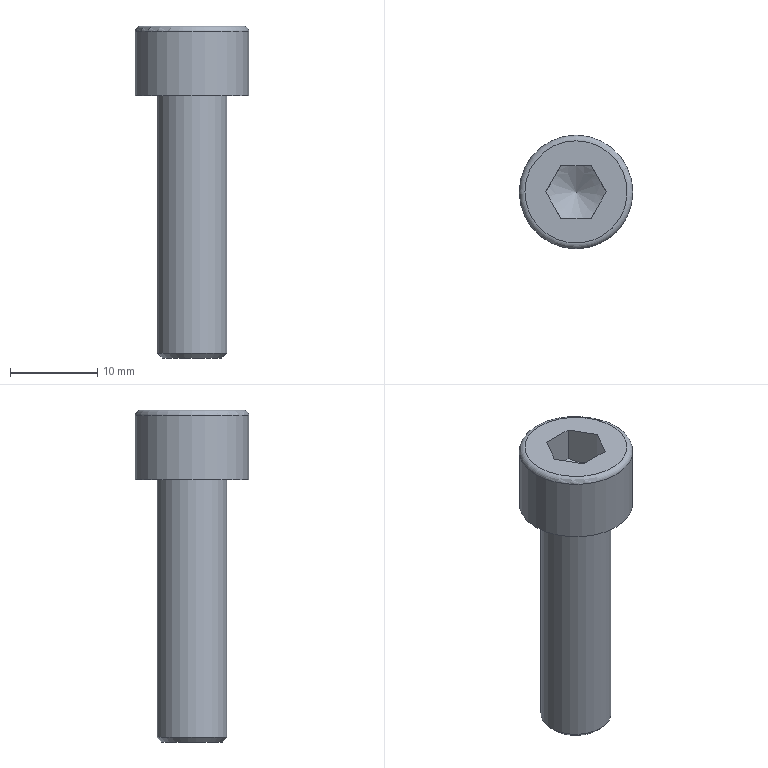Part | STEP file | 1_17 | 1 solid | 14 faces | box 13 x 13 x 38 mm | volume 2414 mm3 | plane 9 | cylinder 2 | cone 2 | torus 1 | commonest cylinder face diameters 8 x1 13 x1
STEP:
#1=CARTESIAN_POINT('',(0.,0.,0.));
#2=DIRECTION('',(0.,0.,1.));
#3=DIRECTION('',(1.,0.,0.));
#4=AXIS2_PLACEMENT_3D('',#1,#2,#3);
#5=CARTESIAN_POINT('',(0.,-6.5,-0.000000001));
#6=VERTEX_POINT('',#5);
#7=CARTESIAN_POINT('',(0.,0.,-0.000000001));
#8=DIRECTION('',(0.,0.,1.));
#9=DIRECTION('',(1.,0.,0.));
#10=AXIS2_PLACEMENT_3D('',#7,#8,#9);
#11=CIRCLE('',#10,6.5);
#12=CARTESIAN_POINT('',(0.,0.,3.675));
#13=DIRECTION('',(0.,0.,1.));
#14=DIRECTION('',(0.,-1.,0.));
#15=AXIS2_PLACEMENT_3D('',#12,#13,#14);
#16=CYLINDRICAL_SURFACE('',#15,6.5);
#17=CARTESIAN_POINT('',(-4.712,-3.675));
#18=DIRECTION('',(1.,0.));
#19=VECTOR('',#18,1.);
#20=LINE('',#17,#19);
#21=(GEOMETRIC_REPRESENTATION_CONTEXT(2)PARAMETRIC_REPRESENTATION_CONTEXT()REPRESENTATION_CONTEXT('',''));
#22=DEFINITIONAL_REPRESENTATION('',(#20),#21);
#23=PCURVE('',#16,#22);
#24=CARTESIAN_POINT('',(0.,3.25,0.));
#25=DIRECTION('',(0.,0.,-1.));
#26=DIRECTION('',(-1.,0.,0.));
#27=AXIS2_PLACEMENT_3D('',#24,#25,#26);
#28=PLANE('',#27);
#29=CARTESIAN_POINT('',(-6.5,-3.25));
#30=CARTESIAN_POINT('',(-6.5,8.008));
#31=CARTESIAN_POINT('',(3.25,2.379));
#32=CARTESIAN_POINT('',(13.,-3.25));
#33=CARTESIAN_POINT('',(3.25,-8.879));
#34=CARTESIAN_POINT('',(-6.5,-14.508));
#35=CARTESIAN_POINT('',(-6.5,-3.25));
#36=(BOUNDED_CURVE()B_SPLINE_CURVE(2,(#29,#30,#31,#32,#33,#34,#35),.UNSPECIFIED.,.T.,.F.)B_SPLINE_CURVE_WITH_KNOTS((1,2,2,2,2,1),(-2.094,0.,2.094,4.189,6.283,8.378),.UNSPECIFIED.)CURVE()GEOMETRIC_REPRESENTATION_ITEM()RATIONAL_B_SPLINE_CURVE((1.,0.5,1.,0.5,1.,0.5,1.))REPRESENTATION_ITEM(''));
#37=(GEOMETRIC_REPRESENTATION_CONTEXT(2)PARAMETRIC_REPRESENTATION_CONTEXT()REPRESENTATION_CONTEXT('',''));
#38=DEFINITIONAL_REPRESENTATION('',(#36),#37);
#39=PCURVE('',#28,#38);
#40=SURFACE_CURVE('',#11,(#23,#39),.PCURVE_S1.);
#41=EDGE_CURVE('',#6,#6,#40,.T.);
#42=ORIENTED_EDGE('',*,*,#41,.T.);
#43=CARTESIAN_POINT('',(0.,-6.5,7.35));
#44=VERTEX_POINT('',#43);
#45=CARTESIAN_POINT('',(0.,-6.5,-0.000000001));
#46=CARTESIAN_POINT('',(0.,-6.5,7.35));
#47=B_SPLINE_CURVE_WITH_KNOTS('',1,(#45,#46),.UNSPECIFIED.,.F.,.F.,(2,2),(-3.675,3.675),.PIECEWISE_BEZIER_KNOTS.);
#48=CARTESIAN_POINT('',(6.283,0.));
#49=DIRECTION('',(0.,1.));
#50=VECTOR('',#49,1.);
#51=LINE('',#48,#50);
#52=(GEOMETRIC_REPRESENTATION_CONTEXT(2)PARAMETRIC_REPRESENTATION_CONTEXT()REPRESENTATION_CONTEXT('',''));
#53=DEFINITIONAL_REPRESENTATION('',(#51),#52);
#54=PCURVE('',#16,#53);
#55=CARTESIAN_POINT('',(0.,0.));
#56=DIRECTION('',(0.,1.));
#57=VECTOR('',#56,1.);
#58=LINE('',#55,#57);
#59=(GEOMETRIC_REPRESENTATION_CONTEXT(2)PARAMETRIC_REPRESENTATION_CONTEXT()REPRESENTATION_CONTEXT('',''));
#60=DEFINITIONAL_REPRESENTATION('',(#58),#59);
#61=PCURVE('',#16,#60);
#62=SEAM_CURVE('',#47,(#54,#61),.PCURVE_S1.);
#63=EDGE_CURVE('',#6,#44,#62,.T.);
#64=ORIENTED_EDGE('',*,*,#63,.T.);
#65=CARTESIAN_POINT('',(-6.5,0.,7.35));
#66=VERTEX_POINT('',#65);
#67=CARTESIAN_POINT('',(0.,0.,7.35));
#68=DIRECTION('',(0.,0.,-1.));
#69=DIRECTION('',(0.,-1.,0.));
#70=AXIS2_PLACEMENT_3D('',#67,#68,#69);
#71=CIRCLE('',#70,6.5);
#72=CARTESIAN_POINT('',(12.566,3.675));
#73=DIRECTION('',(-1.,0.));
#74=VECTOR('',#73,1.);
#75=LINE('',#72,#74);
#76=(GEOMETRIC_REPRESENTATION_CONTEXT(2)PARAMETRIC_REPRESENTATION_CONTEXT()REPRESENTATION_CONTEXT('',''));
#77=DEFINITIONAL_REPRESENTATION('',(#75),#76);
#78=PCURVE('',#16,#77);
#79=CARTESIAN_POINT('',(0.,0.,7.35));
#80=DIRECTION('',(0.,0.,-1.));
#81=DIRECTION('',(-1.,0.,0.));
#82=AXIS2_PLACEMENT_3D('',#79,#80,#81);
#83=TOROIDAL_SURFACE('',#82,5.85,0.65);
#84=CARTESIAN_POINT('',(4.712,6.283));
#85=CARTESIAN_POINT('',(4.736,6.283));
#86=CARTESIAN_POINT('',(4.784,6.283));
#87=CARTESIAN_POINT('',(4.855,6.283));
#88=CARTESIAN_POINT('',(4.927,6.283));
#89=CARTESIAN_POINT('',(4.998,6.283));
#90=CARTESIAN_POINT('',(5.069,6.283));
#91=CARTESIAN_POINT('',(5.141,6.283));
#92=CARTESIAN_POINT('',(5.212,6.283));
#93=CARTESIAN_POINT('',(5.284,6.283));
#94=CARTESIAN_POINT('',(5.355,6.283));
#95=CARTESIAN_POINT('',(5.426,6.283));
#96=CARTESIAN_POINT('',(5.498,6.283));
#97=CARTESIAN_POINT('',(5.569,6.283));
#98=CARTESIAN_POINT('',(5.641,6.283));
#99=CARTESIAN_POINT('',(5.712,6.283));
#100=CARTESIAN_POINT('',(5.783,6.283));
#101=CARTESIAN_POINT('',(5.855,6.283));
#102=CARTESIAN_POINT('',(5.926,6.283));
#103=CARTESIAN_POINT('',(5.998,6.283));
#104=CARTESIAN_POINT('',(6.069,6.283));
#105=CARTESIAN_POINT('',(6.14,6.283));
#106=CARTESIAN_POINT('',(6.212,6.283));
#107=CARTESIAN_POINT('',(6.259,6.283));
#108=CARTESIAN_POINT('',(6.283,6.283));
#109=B_SPLINE_CURVE_WITH_KNOTS('',3,(#84,#85,#86,#87,#88,#89,#90,#91,#92,#93,#94,#95,#96,#97,#98,#99,#100,#101,#102,#103,#104,#105,#106,#107,#108),.UNSPECIFIED.,.F.,.F.,(4,1,1,1,1,1,1,1,1,1,1,1,1,1,1,1,1,1,1,1,1,1,4),(6.283,6.355,6.426,6.497,6.569,6.64,6.712,6.783,6.854,6.926,6.997,7.069,7.14,7.211,7.283,7.354,7.426,7.497,7.568,7.64,7.711,7.783,7.854),.QUASI_UNIFORM_KNOTS.);
#110=(GEOMETRIC_REPRESENTATION_CONTEXT(2)PARAMETRIC_REPRESENTATION_CONTEXT()REPRESENTATION_CONTEXT('',''));
#111=DEFINITIONAL_REPRESENTATION('',(#109),#110);
#112=PCURVE('',#83,#111);
#113=SURFACE_CURVE('',#71,(#78,#112),.PCURVE_S1.);
#114=EDGE_CURVE('',#44,#66,#113,.T.);
#115=ORIENTED_EDGE('',*,*,#114,.T.);
#116=CARTESIAN_POINT('',(6.5,0.,7.35));
#117=VERTEX_POINT('',#116);
#118=CARTESIAN_POINT('',(0.,0.,7.35));
#119=DIRECTION('',(0.,0.,1.));
#120=DIRECTION('',(1.,0.,0.));
#121=AXIS2_PLACEMENT_3D('',#118,#119,#120);
#122=CIRCLE('',#121,6.5);
#123=CARTESIAN_POINT('',(1.571,3.675));
#124=DIRECTION('',(1.,0.));
#125=VECTOR('',#124,1.);
#126=LINE('',#123,#125);
#127=(GEOMETRIC_REPRESENTATION_CONTEXT(2)PARAMETRIC_REPRESENTATION_CONTEXT()REPRESENTATION_CONTEXT('',''));
#128=DEFINITIONAL_REPRESENTATION('',(#126),#127);
#129=PCURVE('',#16,#128);
#130=CARTESIAN_POINT('',(3.142,6.283));
#131=DIRECTION('',(-1.,0.));
#132=VECTOR('',#131,1.);
#133=LINE('',#130,#132);
#134=(GEOMETRIC_REPRESENTATION_CONTEXT(2)PARAMETRIC_REPRESENTATION_CONTEXT()REPRESENTATION_CONTEXT('',''));
#135=DEFINITIONAL_REPRESENTATION('',(#133),#134);
#136=PCURVE('',#83,#135);
#137=SURFACE_CURVE('',#122,(#129,#136),.PCURVE_S1.);
#138=EDGE_CURVE('',#117,#66,#137,.T.);
#139=ORIENTED_EDGE('',*,*,#138,.F.);
#140=CARTESIAN_POINT('',(0.,0.,7.35));
#141=DIRECTION('',(0.,0.,-1.));
#142=DIRECTION('',(0.,-1.,0.));
#143=AXIS2_PLACEMENT_3D('',#140,#141,#142);
#144=CIRCLE('',#143,6.5);
#145=CARTESIAN_POINT('',(6.283,3.675));
#146=DIRECTION('',(-1.,0.));
#147=VECTOR('',#146,1.);
#148=LINE('',#145,#147);
#149=(GEOMETRIC_REPRESENTATION_CONTEXT(2)PARAMETRIC_REPRESENTATION_CONTEXT()REPRESENTATION_CONTEXT('',''));
#150=DEFINITIONAL_REPRESENTATION('',(#148),#149);
#151=PCURVE('',#16,#150);
#152=CARTESIAN_POINT('',(3.142,6.283));
#153=CARTESIAN_POINT('',(3.165,6.283));
#154=CARTESIAN_POINT('',(3.213,6.283));
#155=CARTESIAN_POINT('',(3.284,6.283));
#156=CARTESIAN_POINT('',(3.356,6.283));
#157=CARTESIAN_POINT('',(3.427,6.283));
#158=CARTESIAN_POINT('',(3.499,6.283));
#159=CARTESIAN_POINT('',(3.57,6.283));
#160=CARTESIAN_POINT('',(3.641,6.283));
#161=CARTESIAN_POINT('',(3.713,6.283));
#162=CARTESIAN_POINT('',(3.784,6.283));
#163=CARTESIAN_POINT('',(3.856,6.283));
#164=CARTESIAN_POINT('',(3.927,6.283));
#165=CARTESIAN_POINT('',(3.998,6.283));
#166=CARTESIAN_POINT('',(4.07,6.283));
#167=CARTESIAN_POINT('',(4.141,6.283));
#168=CARTESIAN_POINT('',(4.213,6.283));
#169=CARTESIAN_POINT('',(4.284,6.283));
#170=CARTESIAN_POINT('',(4.355,6.283));
#171=CARTESIAN_POINT('',(4.427,6.283));
#172=CARTESIAN_POINT('',(4.498,6.283));
#173=CARTESIAN_POINT('',(4.57,6.283));
#174=CARTESIAN_POINT('',(4.641,6.283));
#175=CARTESIAN_POINT('',(4.689,6.283));
#176=CARTESIAN_POINT('',(4.712,6.283));
#177=B_SPLINE_CURVE_WITH_KNOTS('',3,(#152,#153,#154,#155,#156,#157,#158,#159,#160,#161,#162,#163,#164,#165,#166,#167,#168,#169,#170,#171,#172,#173,#174,#175,#176),.UNSPECIFIED.,.F.,.F.,(4,1,1,1,1,1,1,1,1,1,1,1,1,1,1,1,1,1,1,1,1,1,4),(4.712,4.784,4.855,4.927,4.998,5.069,5.141,5.212,5.284,5.355,5.426,5.498,5.569,5.641,5.712,5.783,5.855,5.926,5.998,6.069,6.14,6.212,6.283),.QUASI_UNIFORM_KNOTS.);
#178=(GEOMETRIC_REPRESENTATION_CONTEXT(2)PARAMETRIC_REPRESENTATION_CONTEXT()REPRESENTATION_CONTEXT('',''));
#179=DEFINITIONAL_REPRESENTATION('',(#177),#178);
#180=PCURVE('',#83,#179);
#181=SURFACE_CURVE('',#144,(#151,#180),.PCURVE_S1.);
#182=EDGE_CURVE('',#117,#44,#181,.T.);
#183=ORIENTED_EDGE('',*,*,#182,.T.);
#184=ORIENTED_EDGE('',*,*,#63,.F.);
#185=EDGE_LOOP('',(#42,#64,#115,#139,#183,#184));
#186=FACE_BOUND('',#185,.T.);
#187=ADVANCED_FACE('',(#186),#16,.T.);
#188=ORIENTED_EDGE('',*,*,#138,.T.);
#189=CARTESIAN_POINT('',(-5.85,0.,8.));
#190=VERTEX_POINT('',#189);
#191=CARTESIAN_POINT('',(-5.85,0.,8.));
#192=CARTESIAN_POINT('',(-6.024,0.,8.));
#193=CARTESIAN_POINT('',(-6.193,0.,7.945));
#194=CARTESIAN_POINT('',(-6.339,0.,7.839));
#195=CARTESIAN_POINT('',(-6.445,0.,7.693));
#196=CARTESIAN_POINT('',(-6.5,0.,7.524));
#197=CARTESIAN_POINT('',(-6.5,0.,7.35));
#198=(BOUNDED_CURVE()B_SPLINE_CURVE(6,(#191,#192,#193,#194,#195,#196,#197),.UNSPECIFIED.,.F.,.F.)B_SPLINE_CURVE_WITH_KNOTS((7,7),(4.712,6.283),.PIECEWISE_BEZIER_KNOTS.)CURVE()GEOMETRIC_REPRESENTATION_ITEM()RATIONAL_B_SPLINE_CURVE((1.031,1.01,0.9979,0.994,0.9979,1.01,1.031))REPRESENTATION_ITEM(''));
#199=CARTESIAN_POINT('',(0.,0.));
#200=DIRECTION('',(0.,1.));
#201=VECTOR('',#200,1.);
#202=LINE('',#199,#201);
#203=(GEOMETRIC_REPRESENTATION_CONTEXT(2)PARAMETRIC_REPRESENTATION_CONTEXT()REPRESENTATION_CONTEXT('',''));
#204=DEFINITIONAL_REPRESENTATION('',(#202),#203);
#205=PCURVE('',#83,#204);
#206=CARTESIAN_POINT('',(6.283,0.));
#207=DIRECTION('',(0.,1.));
#208=VECTOR('',#207,1.);
#209=LINE('',#206,#208);
#210=(GEOMETRIC_REPRESENTATION_CONTEXT(2)PARAMETRIC_REPRESENTATION_CONTEXT()REPRESENTATION_CONTEXT('',''));
#211=DEFINITIONAL_REPRESENTATION('',(#209),#210);
#212=PCURVE('',#83,#211);
#213=SEAM_CURVE('',#198,(#205,#212),.PCURVE_S1.);
#214=EDGE_CURVE('',#190,#66,#213,.T.);
#215=ORIENTED_EDGE('',*,*,#214,.F.);
#216=CARTESIAN_POINT('',(0.,5.85,8.));
#217=VERTEX_POINT('',#216);
#218=CARTESIAN_POINT('',(0.,0.,8.));
#219=DIRECTION('',(0.,0.,-1.));
#220=DIRECTION('',(1.,0.,0.));
#221=AXIS2_PLACEMENT_3D('',#218,#219,#220);
#222=CIRCLE('',#221,5.85);
#223=CARTESIAN_POINT('',(-3.142,4.712));
#224=DIRECTION('',(1.,0.));
#225=VECTOR('',#224,1.);
#226=LINE('',#223,#225);
#227=(GEOMETRIC_REPRESENTATION_CONTEXT(2)PARAMETRIC_REPRESENTATION_CONTEXT()REPRESENTATION_CONTEXT('',''));
#228=DEFINITIONAL_REPRESENTATION('',(#226),#227);
#229=PCURVE('',#83,#228);
#230=CARTESIAN_POINT('',(0.,2.925,8.));
#231=DIRECTION('',(0.,0.,1.));
#232=DIRECTION('',(1.,0.,0.));
#233=AXIS2_PLACEMENT_3D('',#230,#231,#232);
#234=PLANE('',#233);
#235=CARTESIAN_POINT('',(5.85,-2.925));
#236=CARTESIAN_POINT('',(5.85,-13.057));
#237=CARTESIAN_POINT('',(-2.925,-7.991));
#238=CARTESIAN_POINT('',(-11.7,-2.925));
#239=CARTESIAN_POINT('',(-2.925,2.141));
#240=CARTESIAN_POINT('',(5.85,7.207));
#241=CARTESIAN_POINT('',(5.85,-2.925));
#242=(BOUNDED_CURVE()B_SPLINE_CURVE(2,(#235,#236,#237,#238,#239,#240,#241),.UNSPECIFIED.,.T.,.F.)B_SPLINE_CURVE_WITH_KNOTS((1,2,2,2,2,1),(-2.094,0.,2.094,4.189,6.283,8.378),.UNSPECIFIED.)CURVE()GEOMETRIC_REPRESENTATION_ITEM()RATIONAL_B_SPLINE_CURVE((1.,0.5,1.,0.5,1.,0.5,1.))REPRESENTATION_ITEM(''));
#243=(GEOMETRIC_REPRESENTATION_CONTEXT(2)PARAMETRIC_REPRESENTATION_CONTEXT()REPRESENTATION_CONTEXT('',''));
#244=DEFINITIONAL_REPRESENTATION('',(#242),#243);
#245=PCURVE('',#234,#244);
#246=SURFACE_CURVE('',#222,(#229,#245),.PCURVE_S1.);
#247=EDGE_CURVE('',#190,#217,#246,.T.);
#248=ORIENTED_EDGE('',*,*,#247,.T.);
#249=CARTESIAN_POINT('',(0.,0.,8.));
#250=DIRECTION('',(0.,0.,-1.));
#251=DIRECTION('',(1.,0.,0.));
#252=AXIS2_PLACEMENT_3D('',#249,#250,#251);
#253=CIRCLE('',#252,5.85);
#254=CARTESIAN_POINT('',(-3.142,4.712));
#255=DIRECTION('',(1.,0.));
#256=VECTOR('',#255,1.);
#257=LINE('',#254,#256);
#258=(GEOMETRIC_REPRESENTATION_CONTEXT(2)PARAMETRIC_REPRESENTATION_CONTEXT()REPRESENTATION_CONTEXT('',''));
#259=DEFINITIONAL_REPRESENTATION('',(#257),#258);
#260=PCURVE('',#83,#259);
#261=CARTESIAN_POINT('',(5.85,-2.925));
#262=CARTESIAN_POINT('',(5.85,-13.057));
#263=CARTESIAN_POINT('',(-2.925,-7.991));
#264=CARTESIAN_POINT('',(-11.7,-2.925));
#265=CARTESIAN_POINT('',(-2.925,2.141));
#266=CARTESIAN_POINT('',(5.85,7.207));
#267=CARTESIAN_POINT('',(5.85,-2.925));
#268=(BOUNDED_CURVE()B_SPLINE_CURVE(2,(#261,#262,#263,#264,#265,#266,#267),.UNSPECIFIED.,.T.,.F.)B_SPLINE_CURVE_WITH_KNOTS((1,2,2,2,2,1),(-2.094,0.,2.094,4.189,6.283,8.378),.UNSPECIFIED.)CURVE()GEOMETRIC_REPRESENTATION_ITEM()RATIONAL_B_SPLINE_CURVE((1.,0.5,1.,0.5,1.,0.5,1.))REPRESENTATION_ITEM(''));
#269=(GEOMETRIC_REPRESENTATION_CONTEXT(2)PARAMETRIC_REPRESENTATION_CONTEXT()REPRESENTATION_CONTEXT('',''));
#270=DEFINITIONAL_REPRESENTATION('',(#268),#269);
#271=PCURVE('',#234,#270);
#272=SURFACE_CURVE('',#253,(#260,#271),.PCURVE_S1.);
#273=EDGE_CURVE('',#217,#190,#272,.T.);
#274=ORIENTED_EDGE('',*,*,#273,.T.);
#275=ORIENTED_EDGE('',*,*,#214,.T.);
#276=ORIENTED_EDGE('',*,*,#114,.F.);
#277=ORIENTED_EDGE('',*,*,#182,.F.);
#278=EDGE_LOOP('',(#188,#215,#248,#274,#275,#276,#277));
#279=FACE_BOUND('',#278,.T.);
#280=ADVANCED_FACE('',(#279),#83,.T.);
#281=ORIENTED_EDGE('',*,*,#41,.F.);
#282=EDGE_LOOP('',(#281));
#283=FACE_BOUND('',#282,.T.);
#284=CARTESIAN_POINT('',(0.,-4.,0.));
#285=VERTEX_POINT('',#284);
#286=CARTESIAN_POINT('',(0.,0.,0.));
#287=DIRECTION('',(0.,0.,1.));
#288=DIRECTION('',(0.,1.,0.));
#289=AXIS2_PLACEMENT_3D('',#286,#287,#288);
#290=CIRCLE('',#289,4.);
#291=CARTESIAN_POINT('',(0.,0.75));
#292=CARTESIAN_POINT('',(6.928,0.75));
#293=CARTESIAN_POINT('',(3.464,-5.25));
#294=CARTESIAN_POINT('',(0.,-11.25));
#295=CARTESIAN_POINT('',(-3.464,-5.25));
#296=CARTESIAN_POINT('',(-6.928,0.75));
#297=CARTESIAN_POINT('',(0.,0.75));
#298=(BOUNDED_CURVE()B_SPLINE_CURVE(2,(#291,#292,#293,#294,#295,#296,#297),.UNSPECIFIED.,.T.,.F.)B_SPLINE_CURVE_WITH_KNOTS((1,2,2,2,2,1),(-2.094,0.,2.094,4.189,6.283,8.378),.UNSPECIFIED.)CURVE()GEOMETRIC_REPRESENTATION_ITEM()RATIONAL_B_SPLINE_CURVE((1.,0.5,1.,0.5,1.,0.5,1.))REPRESENTATION_ITEM(''));
#299=(GEOMETRIC_REPRESENTATION_CONTEXT(2)PARAMETRIC_REPRESENTATION_CONTEXT()REPRESENTATION_CONTEXT('',''));
#300=DEFINITIONAL_REPRESENTATION('',(#298),#299);
#301=PCURVE('',#28,#300);
#302=CARTESIAN_POINT('',(0.,0.,-14.229));
#303=DIRECTION('',(0.,0.,1.));
#304=DIRECTION('',(0.,-1.,0.));
#305=AXIS2_PLACEMENT_3D('',#302,#303,#304);
#306=CYLINDRICAL_SURFACE('',#305,4.);
#307=CARTESIAN_POINT('',(-3.142,14.229));
#308=DIRECTION('',(1.,0.));
#309=VECTOR('',#308,1.);
#310=LINE('',#307,#309);
#311=(GEOMETRIC_REPRESENTATION_CONTEXT(2)PARAMETRIC_REPRESENTATION_CONTEXT()REPRESENTATION_CONTEXT('',''));
#312=DEFINITIONAL_REPRESENTATION('',(#310),#311);
#313=PCURVE('',#306,#312);
#314=SURFACE_CURVE('',#290,(#301,#313),.PCURVE_S1.);
#315=EDGE_CURVE('',#285,#285,#314,.T.);
#316=ORIENTED_EDGE('',*,*,#315,.T.);
#317=EDGE_LOOP('',(#316));
#318=FACE_BOUND('',#317,.T.);
#319=ADVANCED_FACE('',(#283,#318),#28,.T.);
#320=ORIENTED_EDGE('',*,*,#273,.F.);
#321=ORIENTED_EDGE('',*,*,#247,.F.);
#322=EDGE_LOOP('',(#320,#321));
#323=FACE_BOUND('',#322,.T.);
#324=CARTESIAN_POINT('',(-1.732,-3.,8.));
#325=VERTEX_POINT('',#324);
#326=CARTESIAN_POINT('',(-3.464,0.,8.));
#327=VERTEX_POINT('',#326);
#328=CARTESIAN_POINT('',(-1.732,-3.,8.));
#329=DIRECTION('',(-0.5,0.866,0.));
#330=VECTOR('',#329,1.);
#331=LINE('',#328,#330);
#332=CARTESIAN_POINT('',(-1.732,-5.925));
#333=DIRECTION('',(-0.5,0.866));
#334=VECTOR('',#333,1.);
#335=LINE('',#332,#334);
#336=(GEOMETRIC_REPRESENTATION_CONTEXT(2)PARAMETRIC_REPRESENTATION_CONTEXT()REPRESENTATION_CONTEXT('',''));
#337=DEFINITIONAL_REPRESENTATION('',(#335),#336);
#338=PCURVE('',#234,#337);
#339=CARTESIAN_POINT('',(-3.464,0.,8.));
#340=DIRECTION('',(-0.866,-0.5,0.));
#341=DIRECTION('',(0.,0.,1.));
#342=AXIS2_PLACEMENT_3D('',#339,#340,#341);
#343=PLANE('',#342);
#344=CARTESIAN_POINT('',(0.,-3.464));
#345=DIRECTION('',(0.,1.));
#346=VECTOR('',#345,1.);
#347=LINE('',#344,#346);
#348=(GEOMETRIC_REPRESENTATION_CONTEXT(2)PARAMETRIC_REPRESENTATION_CONTEXT()REPRESENTATION_CONTEXT('',''));
#349=DEFINITIONAL_REPRESENTATION('',(#347),#348);
#350=PCURVE('',#343,#349);
#351=SURFACE_CURVE('',#331,(#338,#350),.PCURVE_S1.);
#352=EDGE_CURVE('',#325,#327,#351,.T.);
#353=ORIENTED_EDGE('',*,*,#352,.T.);
#354=CARTESIAN_POINT('',(-1.732,3.,8.));
#355=VERTEX_POINT('',#354);
#356=CARTESIAN_POINT('',(-3.464,0.,8.));
#357=DIRECTION('',(0.5,0.866,0.));
#358=VECTOR('',#357,1.);
#359=LINE('',#356,#358);
#360=CARTESIAN_POINT('',(-3.464,-2.925));
#361=DIRECTION('',(0.5,0.866));
#362=VECTOR('',#361,1.);
#363=LINE('',#360,#362);
#364=(GEOMETRIC_REPRESENTATION_CONTEXT(2)PARAMETRIC_REPRESENTATION_CONTEXT()REPRESENTATION_CONTEXT('',''));
#365=DEFINITIONAL_REPRESENTATION('',(#363),#364);
#366=PCURVE('',#234,#365);
#367=CARTESIAN_POINT('',(-1.732,3.,8.));
#368=DIRECTION('',(-0.866,0.5,0.));
#369=DIRECTION('',(0.,0.,1.));
#370=AXIS2_PLACEMENT_3D('',#367,#368,#369);
#371=PLANE('',#370);
#372=CARTESIAN_POINT('',(0.,-3.464));
#373=DIRECTION('',(0.,1.));
#374=VECTOR('',#373,1.);
#375=LINE('',#372,#374);
#376=(GEOMETRIC_REPRESENTATION_CONTEXT(2)PARAMETRIC_REPRESENTATION_CONTEXT()REPRESENTATION_CONTEXT('',''));
#377=DEFINITIONAL_REPRESENTATION('',(#375),#376);
#378=PCURVE('',#371,#377);
#379=SURFACE_CURVE('',#359,(#366,#378),.PCURVE_S1.);
#380=EDGE_CURVE('',#327,#355,#379,.T.);
#381=ORIENTED_EDGE('',*,*,#380,.T.);
#382=CARTESIAN_POINT('',(1.732,3.,8.));
#383=VERTEX_POINT('',#382);
#384=CARTESIAN_POINT('',(-1.732,3.,8.));
#385=DIRECTION('',(1.,0.,0.));
#386=VECTOR('',#385,1.);
#387=LINE('',#384,#386);
#388=CARTESIAN_POINT('',(-1.732,0.075));
#389=DIRECTION('',(1.,0.));
#390=VECTOR('',#389,1.);
#391=LINE('',#388,#390);
#392=(GEOMETRIC_REPRESENTATION_CONTEXT(2)PARAMETRIC_REPRESENTATION_CONTEXT()REPRESENTATION_CONTEXT('',''));
#393=DEFINITIONAL_REPRESENTATION('',(#391),#392);
#394=PCURVE('',#234,#393);
#395=CARTESIAN_POINT('',(1.732,3.,8.));
#396=DIRECTION('',(0.,1.,0.));
#397=DIRECTION('',(0.,0.,1.));
#398=AXIS2_PLACEMENT_3D('',#395,#396,#397);
#399=PLANE('',#398);
#400=CARTESIAN_POINT('',(0.,-3.464));
#401=DIRECTION('',(0.,1.));
#402=VECTOR('',#401,1.);
#403=LINE('',#400,#402);
#404=(GEOMETRIC_REPRESENTATION_CONTEXT(2)PARAMETRIC_REPRESENTATION_CONTEXT()REPRESENTATION_CONTEXT('',''));
#405=DEFINITIONAL_REPRESENTATION('',(#403),#404);
#406=PCURVE('',#399,#405);
#407=SURFACE_CURVE('',#387,(#394,#406),.PCURVE_S1.);
#408=EDGE_CURVE('',#355,#383,#407,.T.);
#409=ORIENTED_EDGE('',*,*,#408,.T.);
#410=CARTESIAN_POINT('',(3.464,0.,8.));
#411=VERTEX_POINT('',#410);
#412=CARTESIAN_POINT('',(1.732,3.,8.));
#413=DIRECTION('',(0.5,-0.866,0.));
#414=VECTOR('',#413,1.);
#415=LINE('',#412,#414);
#416=CARTESIAN_POINT('',(1.732,0.075));
#417=DIRECTION('',(0.5,-0.866));
#418=VECTOR('',#417,1.);
#419=LINE('',#416,#418);
#420=(GEOMETRIC_REPRESENTATION_CONTEXT(2)PARAMETRIC_REPRESENTATION_CONTEXT()REPRESENTATION_CONTEXT('',''));
#421=DEFINITIONAL_REPRESENTATION('',(#419),#420);
#422=PCURVE('',#234,#421);
#423=CARTESIAN_POINT('',(3.464,0.,8.));
#424=DIRECTION('',(0.866,0.5,0.));
#425=DIRECTION('',(0.,0.,-1.));
#426=AXIS2_PLACEMENT_3D('',#423,#424,#425);
#427=PLANE('',#426);
#428=CARTESIAN_POINT('',(0.,3.464));
#429=DIRECTION('',(0.,-1.));
#430=VECTOR('',#429,1.);
#431=LINE('',#428,#430);
#432=(GEOMETRIC_REPRESENTATION_CONTEXT(2)PARAMETRIC_REPRESENTATION_CONTEXT()REPRESENTATION_CONTEXT('',''));
#433=DEFINITIONAL_REPRESENTATION('',(#431),#432);
#434=PCURVE('',#427,#433);
#435=SURFACE_CURVE('',#415,(#422,#434),.PCURVE_S1.);
#436=EDGE_CURVE('',#383,#411,#435,.T.);
#437=ORIENTED_EDGE('',*,*,#436,.T.);
#438=CARTESIAN_POINT('',(1.732,-3.,8.));
#439=VERTEX_POINT('',#438);
#440=CARTESIAN_POINT('',(3.464,0.,8.));
#441=DIRECTION('',(-0.5,-0.866,0.));
#442=VECTOR('',#441,1.);
#443=LINE('',#440,#442);
#444=CARTESIAN_POINT('',(3.464,-2.925));
#445=DIRECTION('',(-0.5,-0.866));
#446=VECTOR('',#445,1.);
#447=LINE('',#444,#446);
#448=(GEOMETRIC_REPRESENTATION_CONTEXT(2)PARAMETRIC_REPRESENTATION_CONTEXT()REPRESENTATION_CONTEXT('',''));
#449=DEFINITIONAL_REPRESENTATION('',(#447),#448);
#450=PCURVE('',#234,#449);
#451=CARTESIAN_POINT('',(1.732,-3.,8.));
#452=DIRECTION('',(0.866,-0.5,0.));
#453=DIRECTION('',(0.,0.,-1.));
#454=AXIS2_PLACEMENT_3D('',#451,#452,#453);
#455=PLANE('',#454);
#456=CARTESIAN_POINT('',(0.,3.464));
#457=DIRECTION('',(0.,-1.));
#458=VECTOR('',#457,1.);
#459=LINE('',#456,#458);
#460=(GEOMETRIC_REPRESENTATION_CONTEXT(2)PARAMETRIC_REPRESENTATION_CONTEXT()REPRESENTATION_CONTEXT('',''));
#461=DEFINITIONAL_REPRESENTATION('',(#459),#460);
#462=PCURVE('',#455,#461);
#463=SURFACE_CURVE('',#443,(#450,#462),.PCURVE_S1.);
#464=EDGE_CURVE('',#411,#439,#463,.T.);
#465=ORIENTED_EDGE('',*,*,#464,.T.);
#466=CARTESIAN_POINT('',(1.732,-3.,8.));
#467=DIRECTION('',(-1.,0.,0.));
#468=VECTOR('',#467,1.);
#469=LINE('',#466,#468);
#470=CARTESIAN_POINT('',(1.732,-5.925));
#471=DIRECTION('',(-1.,0.));
#472=VECTOR('',#471,1.);
#473=LINE('',#470,#472);
#474=(GEOMETRIC_REPRESENTATION_CONTEXT(2)PARAMETRIC_REPRESENTATION_CONTEXT()REPRESENTATION_CONTEXT('',''));
#475=DEFINITIONAL_REPRESENTATION('',(#473),#474);
#476=PCURVE('',#234,#475);
#477=CARTESIAN_POINT('',(-1.732,-3.,8.));
#478=DIRECTION('',(0.,-1.,0.));
#479=DIRECTION('',(0.,0.,-1.));
#480=AXIS2_PLACEMENT_3D('',#477,#478,#479);
#481=PLANE('',#480);
#482=CARTESIAN_POINT('',(0.,3.464));
#483=DIRECTION('',(0.,-1.));
#484=VECTOR('',#483,1.);
#485=LINE('',#482,#484);
#486=(GEOMETRIC_REPRESENTATION_CONTEXT(2)PARAMETRIC_REPRESENTATION_CONTEXT()REPRESENTATION_CONTEXT('',''));
#487=DEFINITIONAL_REPRESENTATION('',(#485),#486);
#488=PCURVE('',#481,#487);
#489=SURFACE_CURVE('',#469,(#476,#488),.PCURVE_S1.);
#490=EDGE_CURVE('',#439,#325,#489,.T.);
#491=ORIENTED_EDGE('',*,*,#490,.T.);
#492=EDGE_LOOP('',(#353,#381,#409,#437,#465,#491));
#493=FACE_BOUND('',#492,.T.);
#494=ADVANCED_FACE('',(#323,#493),#234,.T.);
#495=CARTESIAN_POINT('',(0.,-4.,-29.459));
#496=VERTEX_POINT('',#495);
#497=CARTESIAN_POINT('',(0.,0.,-29.459));
#498=DIRECTION('',(0.,0.,1.));
#499=DIRECTION('',(1.,0.,0.));
#500=AXIS2_PLACEMENT_3D('',#497,#498,#499);
#501=CIRCLE('',#500,4.);
#502=CARTESIAN_POINT('',(-4.712,-15.229));
#503=DIRECTION('',(1.,0.));
#504=VECTOR('',#503,1.);
#505=LINE('',#502,#504);
#506=(GEOMETRIC_REPRESENTATION_CONTEXT(2)PARAMETRIC_REPRESENTATION_CONTEXT()REPRESENTATION_CONTEXT('',''));
#507=DEFINITIONAL_REPRESENTATION('',(#505),#506);
#508=PCURVE('',#306,#507);
#509=CARTESIAN_POINT('',(0.,0.,-29.729));
#510=DIRECTION('',(0.,0.,1.));
#511=DIRECTION('',(0.,-1.,0.));
#512=AXIS2_PLACEMENT_3D('',#509,#510,#511);
#513=CONICAL_SURFACE('',#512,3.729,0.7854);
#514=CARTESIAN_POINT('',(-4.712,0.2706));
#515=DIRECTION('',(1.,0.));
#516=VECTOR('',#515,1.);
#517=LINE('',#514,#516);
#518=(GEOMETRIC_REPRESENTATION_CONTEXT(2)PARAMETRIC_REPRESENTATION_CONTEXT()REPRESENTATION_CONTEXT('',''));
#519=DEFINITIONAL_REPRESENTATION('',(#517),#518);
#520=PCURVE('',#513,#519);
#521=SURFACE_CURVE('',#501,(#508,#520),.PCURVE_S1.);
#522=EDGE_CURVE('',#496,#496,#521,.T.);
#523=ORIENTED_EDGE('',*,*,#522,.T.);
#524=CARTESIAN_POINT('',(0.,-4.,-29.459));
#525=CARTESIAN_POINT('',(0.,-4.,0.));
#526=B_SPLINE_CURVE_WITH_KNOTS('',1,(#524,#525),.UNSPECIFIED.,.F.,.F.,(2,2),(-15.229,14.229),.PIECEWISE_BEZIER_KNOTS.);
#527=CARTESIAN_POINT('',(6.283,0.));
#528=DIRECTION('',(0.,1.));
#529=VECTOR('',#528,1.);
#530=LINE('',#527,#529);
#531=(GEOMETRIC_REPRESENTATION_CONTEXT(2)PARAMETRIC_REPRESENTATION_CONTEXT()REPRESENTATION_CONTEXT('',''));
#532=DEFINITIONAL_REPRESENTATION('',(#530),#531);
#533=PCURVE('',#306,#532);
#534=CARTESIAN_POINT('',(0.,0.));
#535=DIRECTION('',(0.,1.));
#536=VECTOR('',#535,1.);
#537=LINE('',#534,#536);
#538=(GEOMETRIC_REPRESENTATION_CONTEXT(2)PARAMETRIC_REPRESENTATION_CONTEXT()REPRESENTATION_CONTEXT('',''));
#539=DEFINITIONAL_REPRESENTATION('',(#537),#538);
#540=PCURVE('',#306,#539);
#541=SEAM_CURVE('',#526,(#533,#540),.PCURVE_S1.);
#542=EDGE_CURVE('',#496,#285,#541,.T.);
#543=ORIENTED_EDGE('',*,*,#542,.T.);
#544=ORIENTED_EDGE('',*,*,#315,.F.);
#545=ORIENTED_EDGE('',*,*,#542,.F.);
#546=EDGE_LOOP('',(#523,#543,#544,#545));
#547=FACE_BOUND('',#546,.T.);
#548=ADVANCED_FACE('',(#547),#306,.T.);
#549=CARTESIAN_POINT('',(-1.732,-3.,4.));
#550=VERTEX_POINT('',#549);
#551=CARTESIAN_POINT('',(-3.464,0.,4.));
#552=VERTEX_POINT('',#551);
#553=CARTESIAN_POINT('',(3.276,-11.673,9.));
#554=CARTESIAN_POINT('',(-2.598,-1.5,2.429));
#555=CARTESIAN_POINT('',(-8.472,8.673,9.));
#556=(BOUNDED_CURVE()B_SPLINE_CURVE(2,(#553,#554,#555),.UNSPECIFIED.,.F.,.F.)B_SPLINE_CURVE_WITH_KNOTS((3,3),(0.,2.575),.PIECEWISE_BEZIER_KNOTS.)CURVE()GEOMETRIC_REPRESENTATION_ITEM()RATIONAL_B_SPLINE_CURVE((1.,4.041,1.))REPRESENTATION_ITEM(''));
#557=CARTESIAN_POINT('',(1.,-13.479));
#558=CARTESIAN_POINT('',(-5.571,-1.732));
#559=CARTESIAN_POINT('',(1.,10.015));
#560=(BOUNDED_CURVE()B_SPLINE_CURVE(2,(#557,#558,#559),.UNSPECIFIED.,.F.,.F.)B_SPLINE_CURVE_WITH_KNOTS((3,3),(0.,2.575),.PIECEWISE_BEZIER_KNOTS.)CURVE()GEOMETRIC_REPRESENTATION_ITEM()RATIONAL_B_SPLINE_CURVE((1.,4.041,1.))REPRESENTATION_ITEM(''));
#561=(GEOMETRIC_REPRESENTATION_CONTEXT(2)PARAMETRIC_REPRESENTATION_CONTEXT()REPRESENTATION_CONTEXT('',''));
#562=DEFINITIONAL_REPRESENTATION('',(#560),#561);
#563=PCURVE('',#343,#562);
#564=CARTESIAN_POINT('',(0.,0.,3.));
#565=DIRECTION('',(0.,0.,1.));
#566=DIRECTION('',(0.,1.,0.));
#567=AXIS2_PLACEMENT_3D('',#564,#565,#566);
#568=CONICAL_SURFACE('',#567,1.732,1.047);
#569=CARTESIAN_POINT('',(2.618,1.));
#570=CARTESIAN_POINT('',(2.603,0.9825));
#571=CARTESIAN_POINT('',(2.572,0.9496));
#572=CARTESIAN_POINT('',(2.526,0.906));
#573=CARTESIAN_POINT('',(2.479,0.8679));
#574=CARTESIAN_POINT('',(2.432,0.835));
#575=CARTESIAN_POINT('',(2.385,0.8069));
#576=CARTESIAN_POINT('',(2.337,0.7835));
#577=CARTESIAN_POINT('',(2.289,0.7645));
#578=CARTESIAN_POINT('',(2.24,0.7499));
#579=CARTESIAN_POINT('',(2.192,0.7396));
#580=CARTESIAN_POINT('',(2.143,0.7334));
#581=CARTESIAN_POINT('',(2.094,0.7314));
#582=CARTESIAN_POINT('',(2.046,0.7334));
#583=CARTESIAN_POINT('',(1.997,0.7396));
#584=CARTESIAN_POINT('',(1.948,0.7499));
#585=CARTESIAN_POINT('',(1.9,0.7645));
#586=CARTESIAN_POINT('',(1.852,0.7835));
#587=CARTESIAN_POINT('',(1.804,0.8069));
#588=CARTESIAN_POINT('',(1.757,0.835));
#589=CARTESIAN_POINT('',(1.709,0.8679));
#590=CARTESIAN_POINT('',(1.663,0.906));
#591=CARTESIAN_POINT('',(1.616,0.9496));
#592=CARTESIAN_POINT('',(1.586,0.9825));
#593=CARTESIAN_POINT('',(1.571,1.));
#594=B_SPLINE_CURVE_WITH_KNOTS('',3,(#569,#570,#571,#572,#573,#574,#575,#576,#577,#578,#579,#580,#581,#582,#583,#584,#585,#586,#587,#588,#589,#590,#591,#592,#593),.UNSPECIFIED.,.F.,.F.,(4,1,1,1,1,1,1,1,1,1,1,1,1,1,1,1,1,1,1,1,1,1,4),(0.8433,0.8837,0.9241,0.9644,1.005,1.045,1.086,1.126,1.166,1.207,1.247,1.287,1.328,1.368,1.409,1.449,1.489,1.53,1.57,1.61,1.651,1.691,1.732),.QUASI_UNIFORM_KNOTS.);
#595=(GEOMETRIC_REPRESENTATION_CONTEXT(2)PARAMETRIC_REPRESENTATION_CONTEXT()REPRESENTATION_CONTEXT('',''));
#596=DEFINITIONAL_REPRESENTATION('',(#594),#595);
#597=PCURVE('',#568,#596);
#598=SURFACE_CURVE('',#556,(#563,#597),.PCURVE_S1.);
#599=EDGE_CURVE('',#550,#552,#598,.T.);
#600=ORIENTED_EDGE('',*,*,#599,.T.);
#601=CARTESIAN_POINT('',(-3.464,0.,8.));
#602=DIRECTION('',(0.,0.,-1.));
#603=VECTOR('',#602,1.);
#604=LINE('',#601,#603);
#605=CARTESIAN_POINT('',(0.,0.));
#606=DIRECTION('',(-1.,0.));
#607=VECTOR('',#606,1.);
#608=LINE('',#605,#607);
#609=(GEOMETRIC_REPRESENTATION_CONTEXT(2)PARAMETRIC_REPRESENTATION_CONTEXT()REPRESENTATION_CONTEXT('',''));
#610=DEFINITIONAL_REPRESENTATION('',(#608),#609);
#611=PCURVE('',#343,#610);
#612=CARTESIAN_POINT('',(0.,-3.464));
#613=DIRECTION('',(-1.,0.));
#614=VECTOR('',#613,1.);
#615=LINE('',#612,#614);
#616=(GEOMETRIC_REPRESENTATION_CONTEXT(2)PARAMETRIC_REPRESENTATION_CONTEXT()REPRESENTATION_CONTEXT('',''));
#617=DEFINITIONAL_REPRESENTATION('',(#615),#616);
#618=PCURVE('',#371,#617);
#619=SURFACE_CURVE('',#604,(#611,#618),.PCURVE_S1.);
#620=EDGE_CURVE('',#327,#552,#619,.T.);
#621=ORIENTED_EDGE('',*,*,#620,.F.);
#622=ORIENTED_EDGE('',*,*,#352,.F.);
#623=CARTESIAN_POINT('',(-1.732,-3.,8.));
#624=DIRECTION('',(0.,0.,-1.));
#625=VECTOR('',#624,1.);
#626=LINE('',#623,#625);
#627=CARTESIAN_POINT('',(0.,-3.464));
#628=DIRECTION('',(-1.,0.));
#629=VECTOR('',#628,1.);
#630=LINE('',#627,#629);
#631=(GEOMETRIC_REPRESENTATION_CONTEXT(2)PARAMETRIC_REPRESENTATION_CONTEXT()REPRESENTATION_CONTEXT('',''));
#632=DEFINITIONAL_REPRESENTATION('',(#630),#631);
#633=PCURVE('',#343,#632);
#634=CARTESIAN_POINT('',(0.,0.));
#635=DIRECTION('',(1.,0.));
#636=VECTOR('',#635,1.);
#637=LINE('',#634,#636);
#638=(GEOMETRIC_REPRESENTATION_CONTEXT(2)PARAMETRIC_REPRESENTATION_CONTEXT()REPRESENTATION_CONTEXT('',''));
#639=DEFINITIONAL_REPRESENTATION('',(#637),#638);
#640=PCURVE('',#481,#639);
#641=SURFACE_CURVE('',#626,(#633,#640),.PCURVE_S1.);
#642=EDGE_CURVE('',#325,#550,#641,.T.);
#643=ORIENTED_EDGE('',*,*,#642,.T.);
#644=EDGE_LOOP('',(#600,#621,#622,#643));
#645=FACE_BOUND('',#644,.T.);
#646=ADVANCED_FACE('',(#645),#343,.F.);
#647=CARTESIAN_POINT('',(-1.732,3.,4.));
#648=VERTEX_POINT('',#647);
#649=CARTESIAN_POINT('',(-8.472,-8.673,9.));
#650=CARTESIAN_POINT('',(-2.598,1.5,2.429));
#651=CARTESIAN_POINT('',(3.276,11.673,9.));
#652=(BOUNDED_CURVE()B_SPLINE_CURVE(2,(#649,#650,#651),.UNSPECIFIED.,.F.,.F.)B_SPLINE_CURVE_WITH_KNOTS((3,3),(0.,2.575),.PIECEWISE_BEZIER_KNOTS.)CURVE()GEOMETRIC_REPRESENTATION_ITEM()RATIONAL_B_SPLINE_CURVE((1.,4.041,1.))REPRESENTATION_ITEM(''));
#653=CARTESIAN_POINT('',(1.,-13.479));
#654=CARTESIAN_POINT('',(-5.571,-1.732));
#655=CARTESIAN_POINT('',(1.,10.015));
#656=(BOUNDED_CURVE()B_SPLINE_CURVE(2,(#653,#654,#655),.UNSPECIFIED.,.F.,.F.)B_SPLINE_CURVE_WITH_KNOTS((3,3),(0.,2.575),.PIECEWISE_BEZIER_KNOTS.)CURVE()GEOMETRIC_REPRESENTATION_ITEM()RATIONAL_B_SPLINE_CURVE((1.,4.041,1.))REPRESENTATION_ITEM(''));
#657=(GEOMETRIC_REPRESENTATION_CONTEXT(2)PARAMETRIC_REPRESENTATION_CONTEXT()REPRESENTATION_CONTEXT('',''));
#658=DEFINITIONAL_REPRESENTATION('',(#656),#657);
#659=PCURVE('',#371,#658);
#660=CARTESIAN_POINT('',(1.571,1.));
#661=CARTESIAN_POINT('',(1.556,0.9825));
#662=CARTESIAN_POINT('',(1.525,0.9496));
#663=CARTESIAN_POINT('',(1.479,0.906));
#664=CARTESIAN_POINT('',(1.432,0.8679));
#665=CARTESIAN_POINT('',(1.385,0.835));
#666=CARTESIAN_POINT('',(1.338,0.8069));
#667=CARTESIAN_POINT('',(1.29,0.7835));
#668=CARTESIAN_POINT('',(1.241,0.7645));
#669=CARTESIAN_POINT('',(1.193,0.7499));
#670=CARTESIAN_POINT('',(1.145,0.7396));
#671=CARTESIAN_POINT('',(1.096,0.7334));
#672=CARTESIAN_POINT('',(1.047,0.7314));
#673=CARTESIAN_POINT('',(0.9985,0.7334));
#674=CARTESIAN_POINT('',(0.9498,0.7396));
#675=CARTESIAN_POINT('',(0.9013,0.7499));
#676=CARTESIAN_POINT('',(0.8529,0.7645));
#677=CARTESIAN_POINT('',(0.8048,0.7835));
#678=CARTESIAN_POINT('',(0.7569,0.8069));
#679=CARTESIAN_POINT('',(0.7094,0.835));
#680=CARTESIAN_POINT('',(0.6622,0.8679));
#681=CARTESIAN_POINT('',(0.6155,0.906));
#682=CARTESIAN_POINT('',(0.5692,0.9496));
#683=CARTESIAN_POINT('',(0.5388,0.9825));
#684=CARTESIAN_POINT('',(0.5236,1.));
#685=B_SPLINE_CURVE_WITH_KNOTS('',3,(#660,#661,#662,#663,#664,#665,#666,#667,#668,#669,#670,#671,#672,#673,#674,#675,#676,#677,#678,#679,#680,#681,#682,#683,#684),.UNSPECIFIED.,.F.,.F.,(4,1,1,1,1,1,1,1,1,1,1,1,1,1,1,1,1,1,1,1,1,1,4),(0.8433,0.8837,0.9241,0.9644,1.005,1.045,1.086,1.126,1.166,1.207,1.247,1.287,1.328,1.368,1.409,1.449,1.489,1.53,1.57,1.61,1.651,1.691,1.732),.QUASI_UNIFORM_KNOTS.);
#686=(GEOMETRIC_REPRESENTATION_CONTEXT(2)PARAMETRIC_REPRESENTATION_CONTEXT()REPRESENTATION_CONTEXT('',''));
#687=DEFINITIONAL_REPRESENTATION('',(#685),#686);
#688=PCURVE('',#568,#687);
#689=SURFACE_CURVE('',#652,(#659,#688),.PCURVE_S1.);
#690=EDGE_CURVE('',#552,#648,#689,.T.);
#691=ORIENTED_EDGE('',*,*,#690,.T.);
#692=CARTESIAN_POINT('',(-1.732,3.,8.));
#693=DIRECTION('',(0.,0.,-1.));
#694=VECTOR('',#693,1.);
#695=LINE('',#692,#694);
#696=CARTESIAN_POINT('',(0.,0.));
#697=DIRECTION('',(-1.,0.));
#698=VECTOR('',#697,1.);
#699=LINE('',#696,#698);
#700=(GEOMETRIC_REPRESENTATION_CONTEXT(2)PARAMETRIC_REPRESENTATION_CONTEXT()REPRESENTATION_CONTEXT('',''));
#701=DEFINITIONAL_REPRESENTATION('',(#699),#700);
#702=PCURVE('',#371,#701);
#703=CARTESIAN_POINT('',(0.,-3.464));
#704=DIRECTION('',(-1.,0.));
#705=VECTOR('',#704,1.);
#706=LINE('',#703,#705);
#707=(GEOMETRIC_REPRESENTATION_CONTEXT(2)PARAMETRIC_REPRESENTATION_CONTEXT()REPRESENTATION_CONTEXT('',''));
#708=DEFINITIONAL_REPRESENTATION('',(#706),#707);
#709=PCURVE('',#399,#708);
#710=SURFACE_CURVE('',#695,(#702,#709),.PCURVE_S1.);
#711=EDGE_CURVE('',#355,#648,#710,.T.);
#712=ORIENTED_EDGE('',*,*,#711,.F.);
#713=ORIENTED_EDGE('',*,*,#380,.F.);
#714=ORIENTED_EDGE('',*,*,#620,.T.);
#715=EDGE_LOOP('',(#691,#712,#713,#714));
#716=FACE_BOUND('',#715,.T.);
#717=ADVANCED_FACE('',(#716),#371,.F.);
#718=CARTESIAN_POINT('',(0.,3.,3.732));
#719=VERTEX_POINT('',#718);
#720=CARTESIAN_POINT('',(-1.732,3.,4.));
#721=CARTESIAN_POINT('',(-1.366,3.,3.894));
#722=CARTESIAN_POINT('',(-1.013,3.,3.813));
#723=CARTESIAN_POINT('',(-0.6709,3.,3.759));
#724=CARTESIAN_POINT('',(-0.3355,3.,3.732));
#725=CARTESIAN_POINT('',(0.,3.,3.732));
#726=B_SPLINE_CURVE_WITH_KNOTS('',5,(#720,#721,#722,#723,#724,#725),.UNSPECIFIED.,.F.,.F.,(6,6),(0.,2.52),.PIECEWISE_BEZIER_KNOTS.);
#727=CARTESIAN_POINT('',(-4.,-3.464));
#728=CARTESIAN_POINT('',(-4.106,-3.098));
#729=CARTESIAN_POINT('',(-4.187,-2.745));
#730=CARTESIAN_POINT('',(-4.241,-2.403));
#731=CARTESIAN_POINT('',(-4.268,-2.068));
#732=CARTESIAN_POINT('',(-4.268,-1.732));
#733=B_SPLINE_CURVE_WITH_KNOTS('',5,(#727,#728,#729,#730,#731,#732),.UNSPECIFIED.,.F.,.F.,(6,6),(0.,2.52),.PIECEWISE_BEZIER_KNOTS.);
#734=(GEOMETRIC_REPRESENTATION_CONTEXT(2)PARAMETRIC_REPRESENTATION_CONTEXT()REPRESENTATION_CONTEXT('',''));
#735=DEFINITIONAL_REPRESENTATION('',(#733),#734);
#736=PCURVE('',#399,#735);
#737=CARTESIAN_POINT('',(0.5236,1.));
#738=CARTESIAN_POINT('',(0.5167,0.992));
#739=CARTESIAN_POINT('',(0.5027,0.9763));
#740=CARTESIAN_POINT('',(0.4813,0.9538));
#741=CARTESIAN_POINT('',(0.4596,0.9324));
#742=CARTESIAN_POINT('',(0.4376,0.912));
#743=CARTESIAN_POINT('',(0.4152,0.8927));
#744=CARTESIAN_POINT('',(0.3926,0.8744));
#745=CARTESIAN_POINT('',(0.3696,0.8573));
#746=CARTESIAN_POINT('',(0.3463,0.8412));
#747=CARTESIAN_POINT('',(0.3228,0.8262));
#748=CARTESIAN_POINT('',(0.299,0.8122));
#749=CARTESIAN_POINT('',(0.2749,0.7994));
#750=CARTESIAN_POINT('',(0.2507,0.7877));
#751=CARTESIAN_POINT('',(0.2262,0.7771));
#752=CARTESIAN_POINT('',(0.2015,0.7676));
#753=CARTESIAN_POINT('',(0.1767,0.7593));
#754=CARTESIAN_POINT('',(0.1517,0.752));
#755=CARTESIAN_POINT('',(0.1266,0.7458));
#756=CARTESIAN_POINT('',(0.1014,0.7408));
#757=CARTESIAN_POINT('',(0.07616,0.7369));
#758=CARTESIAN_POINT('',(0.05081,0.7341));
#759=CARTESIAN_POINT('',(0.02541,0.7324));
#760=CARTESIAN_POINT('',(0.008472,0.7321));
#761=CARTESIAN_POINT('',(0.,0.7321));
#762=B_SPLINE_CURVE_WITH_KNOTS('',3,(#737,#738,#739,#740,#741,#742,#743,#744,#745,#746,#747,#748,#749,#750,#751,#752,#753,#754,#755,#756,#757,#758,#759,#760,#761),.UNSPECIFIED.,.F.,.F.,(4,1,1,1,1,1,1,1,1,1,1,1,1,1,1,1,1,1,1,1,1,1,4),(0.,0.1146,0.2291,0.3437,0.4582,0.5728,0.6873,0.8019,0.9164,1.031,1.146,1.26,1.375,1.489,1.604,1.718,1.833,1.947,2.062,2.177,2.291,2.406,2.52),.QUASI_UNIFORM_KNOTS.);
#763=(GEOMETRIC_REPRESENTATION_CONTEXT(2)PARAMETRIC_REPRESENTATION_CONTEXT()REPRESENTATION_CONTEXT('',''));
#764=DEFINITIONAL_REPRESENTATION('',(#762),#763);
#765=PCURVE('',#568,#764);
#766=SURFACE_CURVE('',#726,(#736,#765),.PCURVE_S1.);
#767=EDGE_CURVE('',#648,#719,#766,.T.);
#768=ORIENTED_EDGE('',*,*,#767,.T.);
#769=CARTESIAN_POINT('',(1.732,3.,4.));
#770=VERTEX_POINT('',#769);
#771=CARTESIAN_POINT('',(0.,3.,3.732));
#772=CARTESIAN_POINT('',(0.3355,3.,3.732));
#773=CARTESIAN_POINT('',(0.6709,3.,3.759));
#774=CARTESIAN_POINT('',(1.013,3.,3.813));
#775=CARTESIAN_POINT('',(1.366,3.,3.894));
#776=CARTESIAN_POINT('',(1.732,3.,4.));
#777=B_SPLINE_CURVE_WITH_KNOTS('',5,(#771,#772,#773,#774,#775,#776),.UNSPECIFIED.,.F.,.F.,(6,6),(0.,2.52),.PIECEWISE_BEZIER_KNOTS.);
#778=CARTESIAN_POINT('',(-4.268,-1.732));
#779=CARTESIAN_POINT('',(-4.268,-1.397));
#780=CARTESIAN_POINT('',(-4.241,-1.061));
#781=CARTESIAN_POINT('',(-4.187,-0.7194));
#782=CARTESIAN_POINT('',(-4.106,-0.3661));
#783=CARTESIAN_POINT('',(-4.,0.));
#784=B_SPLINE_CURVE_WITH_KNOTS('',5,(#778,#779,#780,#781,#782,#783),.UNSPECIFIED.,.F.,.F.,(6,6),(0.,2.52),.PIECEWISE_BEZIER_KNOTS.);
#785=(GEOMETRIC_REPRESENTATION_CONTEXT(2)PARAMETRIC_REPRESENTATION_CONTEXT()REPRESENTATION_CONTEXT('',''));
#786=DEFINITIONAL_REPRESENTATION('',(#784),#785);
#787=PCURVE('',#399,#786);
#788=CARTESIAN_POINT('',(6.283,0.7321));
#789=CARTESIAN_POINT('',(6.275,0.7321));
#790=CARTESIAN_POINT('',(6.258,0.7324));
#791=CARTESIAN_POINT('',(6.232,0.7341));
#792=CARTESIAN_POINT('',(6.207,0.7369));
#793=CARTESIAN_POINT('',(6.182,0.7408));
#794=CARTESIAN_POINT('',(6.157,0.7458));
#795=CARTESIAN_POINT('',(6.131,0.752));
#796=CARTESIAN_POINT('',(6.106,0.7593));
#797=CARTESIAN_POINT('',(6.082,0.7676));
#798=CARTESIAN_POINT('',(6.057,0.7771));
#799=CARTESIAN_POINT('',(6.033,0.7877));
#800=CARTESIAN_POINT('',(6.008,0.7994));
#801=CARTESIAN_POINT('',(5.984,0.8122));
#802=CARTESIAN_POINT('',(5.96,0.8262));
#803=CARTESIAN_POINT('',(5.937,0.8412));
#804=CARTESIAN_POINT('',(5.914,0.8573));
#805=CARTESIAN_POINT('',(5.891,0.8744));
#806=CARTESIAN_POINT('',(5.868,0.8927));
#807=CARTESIAN_POINT('',(5.846,0.912));
#808=CARTESIAN_POINT('',(5.824,0.9324));
#809=CARTESIAN_POINT('',(5.802,0.9538));
#810=CARTESIAN_POINT('',(5.781,0.9763));
#811=CARTESIAN_POINT('',(5.767,0.992));
#812=CARTESIAN_POINT('',(5.76,1.));
#813=B_SPLINE_CURVE_WITH_KNOTS('',3,(#788,#789,#790,#791,#792,#793,#794,#795,#796,#797,#798,#799,#800,#801,#802,#803,#804,#805,#806,#807,#808,#809,#810,#811,#812),.UNSPECIFIED.,.F.,.F.,(4,1,1,1,1,1,1,1,1,1,1,1,1,1,1,1,1,1,1,1,1,1,4),(0.,0.1146,0.2291,0.3437,0.4582,0.5728,0.6873,0.8019,0.9164,1.031,1.146,1.26,1.375,1.489,1.604,1.718,1.833,1.947,2.062,2.177,2.291,2.406,2.52),.QUASI_UNIFORM_KNOTS.);
#814=(GEOMETRIC_REPRESENTATION_CONTEXT(2)PARAMETRIC_REPRESENTATION_CONTEXT()REPRESENTATION_CONTEXT('',''));
#815=DEFINITIONAL_REPRESENTATION('',(#813),#814);
#816=PCURVE('',#568,#815);
#817=SURFACE_CURVE('',#777,(#787,#816),.PCURVE_S1.);
#818=EDGE_CURVE('',#719,#770,#817,.T.);
#819=ORIENTED_EDGE('',*,*,#818,.T.);
#820=CARTESIAN_POINT('',(1.732,3.,8.));
#821=DIRECTION('',(0.,0.,-1.));
#822=VECTOR('',#821,1.);
#823=LINE('',#820,#822);
#824=CARTESIAN_POINT('',(0.,0.));
#825=DIRECTION('',(-1.,0.));
#826=VECTOR('',#825,1.);
#827=LINE('',#824,#826);
#828=(GEOMETRIC_REPRESENTATION_CONTEXT(2)PARAMETRIC_REPRESENTATION_CONTEXT()REPRESENTATION_CONTEXT('',''));
#829=DEFINITIONAL_REPRESENTATION('',(#827),#828);
#830=PCURVE('',#399,#829);
#831=CARTESIAN_POINT('',(0.,3.464));
#832=DIRECTION('',(1.,0.));
#833=VECTOR('',#832,1.);
#834=LINE('',#831,#833);
#835=(GEOMETRIC_REPRESENTATION_CONTEXT(2)PARAMETRIC_REPRESENTATION_CONTEXT()REPRESENTATION_CONTEXT('',''));
#836=DEFINITIONAL_REPRESENTATION('',(#834),#835);
#837=PCURVE('',#427,#836);
#838=SURFACE_CURVE('',#823,(#830,#837),.PCURVE_S1.);
#839=EDGE_CURVE('',#383,#770,#838,.T.);
#840=ORIENTED_EDGE('',*,*,#839,.F.);
#841=ORIENTED_EDGE('',*,*,#408,.F.);
#842=ORIENTED_EDGE('',*,*,#711,.T.);
#843=EDGE_LOOP('',(#768,#819,#840,#841,#842));
#844=FACE_BOUND('',#843,.T.);
#845=ADVANCED_FACE('',(#844),#399,.F.);
#846=CARTESIAN_POINT('',(3.464,0.,4.));
#847=VERTEX_POINT('',#846);
#848=CARTESIAN_POINT('',(-3.276,11.673,9.));
#849=CARTESIAN_POINT('',(2.598,1.5,2.429));
#850=CARTESIAN_POINT('',(8.472,-8.673,9.));
#851=(BOUNDED_CURVE()B_SPLINE_CURVE(2,(#848,#849,#850),.UNSPECIFIED.,.F.,.F.)B_SPLINE_CURVE_WITH_KNOTS((3,3),(0.,2.575),.PIECEWISE_BEZIER_KNOTS.)CURVE()GEOMETRIC_REPRESENTATION_ITEM()RATIONAL_B_SPLINE_CURVE((1.,4.041,1.))REPRESENTATION_ITEM(''));
#852=CARTESIAN_POINT('',(-1.,13.479));
#853=CARTESIAN_POINT('',(5.571,1.732));
#854=CARTESIAN_POINT('',(-1.,-10.015));
#855=(BOUNDED_CURVE()B_SPLINE_CURVE(2,(#852,#853,#854),.UNSPECIFIED.,.F.,.F.)B_SPLINE_CURVE_WITH_KNOTS((3,3),(0.,2.575),.PIECEWISE_BEZIER_KNOTS.)CURVE()GEOMETRIC_REPRESENTATION_ITEM()RATIONAL_B_SPLINE_CURVE((1.,4.041,1.))REPRESENTATION_ITEM(''));
#856=(GEOMETRIC_REPRESENTATION_CONTEXT(2)PARAMETRIC_REPRESENTATION_CONTEXT()REPRESENTATION_CONTEXT('',''));
#857=DEFINITIONAL_REPRESENTATION('',(#855),#856);
#858=PCURVE('',#427,#857);
#859=CARTESIAN_POINT('',(5.76,1.));
#860=CARTESIAN_POINT('',(5.744,0.9825));
#861=CARTESIAN_POINT('',(5.714,0.9496));
#862=CARTESIAN_POINT('',(5.668,0.906));
#863=CARTESIAN_POINT('',(5.621,0.8679));
#864=CARTESIAN_POINT('',(5.574,0.835));
#865=CARTESIAN_POINT('',(5.526,0.8069));
#866=CARTESIAN_POINT('',(5.478,0.7835));
#867=CARTESIAN_POINT('',(5.43,0.7645));
#868=CARTESIAN_POINT('',(5.382,0.7499));
#869=CARTESIAN_POINT('',(5.333,0.7396));
#870=CARTESIAN_POINT('',(5.285,0.7334));
#871=CARTESIAN_POINT('',(5.236,0.7314));
#872=CARTESIAN_POINT('',(5.187,0.7334));
#873=CARTESIAN_POINT('',(5.139,0.7396));
#874=CARTESIAN_POINT('',(5.09,0.7499));
#875=CARTESIAN_POINT('',(5.042,0.7645));
#876=CARTESIAN_POINT('',(4.994,0.7835));
#877=CARTESIAN_POINT('',(4.946,0.8069));
#878=CARTESIAN_POINT('',(4.898,0.835));
#879=CARTESIAN_POINT('',(4.851,0.8679));
#880=CARTESIAN_POINT('',(4.804,0.906));
#881=CARTESIAN_POINT('',(4.758,0.9496));
#882=CARTESIAN_POINT('',(4.728,0.9825));
#883=CARTESIAN_POINT('',(4.712,1.));
#884=B_SPLINE_CURVE_WITH_KNOTS('',3,(#859,#860,#861,#862,#863,#864,#865,#866,#867,#868,#869,#870,#871,#872,#873,#874,#875,#876,#877,#878,#879,#880,#881,#882,#883),.UNSPECIFIED.,.F.,.F.,(4,1,1,1,1,1,1,1,1,1,1,1,1,1,1,1,1,1,1,1,1,1,4),(0.8433,0.8837,0.9241,0.9644,1.005,1.045,1.086,1.126,1.166,1.207,1.247,1.287,1.328,1.368,1.409,1.449,1.489,1.53,1.57,1.61,1.651,1.691,1.732),.QUASI_UNIFORM_KNOTS.);
#885=(GEOMETRIC_REPRESENTATION_CONTEXT(2)PARAMETRIC_REPRESENTATION_CONTEXT()REPRESENTATION_CONTEXT('',''));
#886=DEFINITIONAL_REPRESENTATION('',(#884),#885);
#887=PCURVE('',#568,#886);
#888=SURFACE_CURVE('',#851,(#858,#887),.PCURVE_S1.);
#889=EDGE_CURVE('',#770,#847,#888,.T.);
#890=ORIENTED_EDGE('',*,*,#889,.T.);
#891=CARTESIAN_POINT('',(3.464,0.,8.));
#892=DIRECTION('',(0.,0.,-1.));
#893=VECTOR('',#892,1.);
#894=LINE('',#891,#893);
#895=CARTESIAN_POINT('',(0.,0.));
#896=DIRECTION('',(1.,0.));
#897=VECTOR('',#896,1.);
#898=LINE('',#895,#897);
#899=(GEOMETRIC_REPRESENTATION_CONTEXT(2)PARAMETRIC_REPRESENTATION_CONTEXT()REPRESENTATION_CONTEXT('',''));
#900=DEFINITIONAL_REPRESENTATION('',(#898),#899);
#901=PCURVE('',#427,#900);
#902=CARTESIAN_POINT('',(0.,3.464));
#903=DIRECTION('',(1.,0.));
#904=VECTOR('',#903,1.);
#905=LINE('',#902,#904);
#906=(GEOMETRIC_REPRESENTATION_CONTEXT(2)PARAMETRIC_REPRESENTATION_CONTEXT()REPRESENTATION_CONTEXT('',''));
#907=DEFINITIONAL_REPRESENTATION('',(#905),#906);
#908=PCURVE('',#455,#907);
#909=SURFACE_CURVE('',#894,(#901,#908),.PCURVE_S1.);
#910=EDGE_CURVE('',#411,#847,#909,.T.);
#911=ORIENTED_EDGE('',*,*,#910,.F.);
#912=ORIENTED_EDGE('',*,*,#436,.F.);
#913=ORIENTED_EDGE('',*,*,#839,.T.);
#914=EDGE_LOOP('',(#890,#911,#912,#913));
#915=FACE_BOUND('',#914,.T.);
#916=ADVANCED_FACE('',(#915),#427,.F.);
#917=CARTESIAN_POINT('',(1.732,-3.,4.));
#918=VERTEX_POINT('',#917);
#919=CARTESIAN_POINT('',(8.472,8.673,9.));
#920=CARTESIAN_POINT('',(2.598,-1.5,2.429));
#921=CARTESIAN_POINT('',(-3.276,-11.673,9.));
#922=(BOUNDED_CURVE()B_SPLINE_CURVE(2,(#919,#920,#921),.UNSPECIFIED.,.F.,.F.)B_SPLINE_CURVE_WITH_KNOTS((3,3),(0.,2.575),.PIECEWISE_BEZIER_KNOTS.)CURVE()GEOMETRIC_REPRESENTATION_ITEM()RATIONAL_B_SPLINE_CURVE((1.,4.041,1.))REPRESENTATION_ITEM(''));
#923=CARTESIAN_POINT('',(-1.,13.479));
#924=CARTESIAN_POINT('',(5.571,1.732));
#925=CARTESIAN_POINT('',(-1.,-10.015));
#926=(BOUNDED_CURVE()B_SPLINE_CURVE(2,(#923,#924,#925),.UNSPECIFIED.,.F.,.F.)B_SPLINE_CURVE_WITH_KNOTS((3,3),(0.,2.575),.PIECEWISE_BEZIER_KNOTS.)CURVE()GEOMETRIC_REPRESENTATION_ITEM()RATIONAL_B_SPLINE_CURVE((1.,4.041,1.))REPRESENTATION_ITEM(''));
#927=(GEOMETRIC_REPRESENTATION_CONTEXT(2)PARAMETRIC_REPRESENTATION_CONTEXT()REPRESENTATION_CONTEXT('',''));
#928=DEFINITIONAL_REPRESENTATION('',(#926),#927);
#929=PCURVE('',#455,#928);
#930=CARTESIAN_POINT('',(4.712,1.));
#931=CARTESIAN_POINT('',(4.697,0.9825));
#932=CARTESIAN_POINT('',(4.667,0.9496));
#933=CARTESIAN_POINT('',(4.621,0.906));
#934=CARTESIAN_POINT('',(4.574,0.8679));
#935=CARTESIAN_POINT('',(4.527,0.835));
#936=CARTESIAN_POINT('',(4.479,0.8069));
#937=CARTESIAN_POINT('',(4.431,0.7835));
#938=CARTESIAN_POINT('',(4.383,0.7645));
#939=CARTESIAN_POINT('',(4.335,0.7499));
#940=CARTESIAN_POINT('',(4.286,0.7396));
#941=CARTESIAN_POINT('',(4.238,0.7334));
#942=CARTESIAN_POINT('',(4.189,0.7314));
#943=CARTESIAN_POINT('',(4.14,0.7334));
#944=CARTESIAN_POINT('',(4.091,0.7396));
#945=CARTESIAN_POINT('',(4.043,0.7499));
#946=CARTESIAN_POINT('',(3.994,0.7645));
#947=CARTESIAN_POINT('',(3.946,0.7835));
#948=CARTESIAN_POINT('',(3.898,0.8069));
#949=CARTESIAN_POINT('',(3.851,0.835));
#950=CARTESIAN_POINT('',(3.804,0.8679));
#951=CARTESIAN_POINT('',(3.757,0.906));
#952=CARTESIAN_POINT('',(3.711,0.9496));
#953=CARTESIAN_POINT('',(3.68,0.9825));
#954=CARTESIAN_POINT('',(3.665,1.));
#955=B_SPLINE_CURVE_WITH_KNOTS('',3,(#930,#931,#932,#933,#934,#935,#936,#937,#938,#939,#940,#941,#942,#943,#944,#945,#946,#947,#948,#949,#950,#951,#952,#953,#954),.UNSPECIFIED.,.F.,.F.,(4,1,1,1,1,1,1,1,1,1,1,1,1,1,1,1,1,1,1,1,1,1,4),(0.8433,0.8837,0.9241,0.9644,1.005,1.045,1.086,1.126,1.166,1.207,1.247,1.287,1.328,1.368,1.409,1.449,1.489,1.53,1.57,1.61,1.651,1.691,1.732),.QUASI_UNIFORM_KNOTS.);
#956=(GEOMETRIC_REPRESENTATION_CONTEXT(2)PARAMETRIC_REPRESENTATION_CONTEXT()REPRESENTATION_CONTEXT('',''));
#957=DEFINITIONAL_REPRESENTATION('',(#955),#956);
#958=PCURVE('',#568,#957);
#959=SURFACE_CURVE('',#922,(#929,#958),.PCURVE_S1.);
#960=EDGE_CURVE('',#847,#918,#959,.T.);
#961=ORIENTED_EDGE('',*,*,#960,.T.);
#962=CARTESIAN_POINT('',(1.732,-3.,8.));
#963=DIRECTION('',(0.,0.,-1.));
#964=VECTOR('',#963,1.);
#965=LINE('',#962,#964);
#966=CARTESIAN_POINT('',(0.,0.));
#967=DIRECTION('',(1.,0.));
#968=VECTOR('',#967,1.);
#969=LINE('',#966,#968);
#970=(GEOMETRIC_REPRESENTATION_CONTEXT(2)PARAMETRIC_REPRESENTATION_CONTEXT()REPRESENTATION_CONTEXT('',''));
#971=DEFINITIONAL_REPRESENTATION('',(#969),#970);
#972=PCURVE('',#455,#971);
#973=CARTESIAN_POINT('',(0.,3.464));
#974=DIRECTION('',(1.,0.));
#975=VECTOR('',#974,1.);
#976=LINE('',#973,#975);
#977=(GEOMETRIC_REPRESENTATION_CONTEXT(2)PARAMETRIC_REPRESENTATION_CONTEXT()REPRESENTATION_CONTEXT('',''));
#978=DEFINITIONAL_REPRESENTATION('',(#976),#977);
#979=PCURVE('',#481,#978);
#980=SURFACE_CURVE('',#965,(#972,#979),.PCURVE_S1.);
#981=EDGE_CURVE('',#439,#918,#980,.T.);
#982=ORIENTED_EDGE('',*,*,#981,.F.);
#983=ORIENTED_EDGE('',*,*,#464,.F.);
#984=ORIENTED_EDGE('',*,*,#910,.T.);
#985=EDGE_LOOP('',(#961,#982,#983,#984));
#986=FACE_BOUND('',#985,.T.);
#987=ADVANCED_FACE('',(#986),#455,.F.);
#988=CARTESIAN_POINT('',(0.,-3.,3.732));
#989=VERTEX_POINT('',#988);
#990=CARTESIAN_POINT('',(1.732,-3.,4.));
#991=CARTESIAN_POINT('',(1.366,-3.,3.894));
#992=CARTESIAN_POINT('',(1.013,-3.,3.813));
#993=CARTESIAN_POINT('',(0.6709,-3.,3.759));
#994=CARTESIAN_POINT('',(0.3355,-3.,3.732));
#995=CARTESIAN_POINT('',(0.,-3.,3.732));
#996=B_SPLINE_CURVE_WITH_KNOTS('',5,(#990,#991,#992,#993,#994,#995),.UNSPECIFIED.,.F.,.F.,(6,6),(0.,2.52),.PIECEWISE_BEZIER_KNOTS.);
#997=CARTESIAN_POINT('',(4.,3.464));
#998=CARTESIAN_POINT('',(4.106,3.098));
#999=CARTESIAN_POINT('',(4.187,2.745));
#1000=CARTESIAN_POINT('',(4.241,2.403));
#1001=CARTESIAN_POINT('',(4.268,2.068));
#1002=CARTESIAN_POINT('',(4.268,1.732));
#1003=B_SPLINE_CURVE_WITH_KNOTS('',5,(#997,#998,#999,#1000,#1001,#1002),.UNSPECIFIED.,.F.,.F.,(6,6),(0.,2.52),.PIECEWISE_BEZIER_KNOTS.);
#1004=(GEOMETRIC_REPRESENTATION_CONTEXT(2)PARAMETRIC_REPRESENTATION_CONTEXT()REPRESENTATION_CONTEXT('',''));
#1005=DEFINITIONAL_REPRESENTATION('',(#1003),#1004);
#1006=PCURVE('',#481,#1005);
#1007=CARTESIAN_POINT('',(3.665,1.));
#1008=CARTESIAN_POINT('',(3.658,0.992));
#1009=CARTESIAN_POINT('',(3.644,0.9763));
#1010=CARTESIAN_POINT('',(3.623,0.9538));
#1011=CARTESIAN_POINT('',(3.601,0.9324));
#1012=CARTESIAN_POINT('',(3.579,0.912));
#1013=CARTESIAN_POINT('',(3.557,0.8927));
#1014=CARTESIAN_POINT('',(3.534,0.8744));
#1015=CARTESIAN_POINT('',(3.511,0.8573));
#1016=CARTESIAN_POINT('',(3.488,0.8412));
#1017=CARTESIAN_POINT('',(3.464,0.8262));
#1018=CARTESIAN_POINT('',(3.441,0.8122));
#1019=CARTESIAN_POINT('',(3.417,0.7994));
#1020=CARTESIAN_POINT('',(3.392,0.7877));
#1021=CARTESIAN_POINT('',(3.368,0.7771));
#1022=CARTESIAN_POINT('',(3.343,0.7676));
#1023=CARTESIAN_POINT('',(3.318,0.7593));
#1024=CARTESIAN_POINT('',(3.293,0.752));
#1025=CARTESIAN_POINT('',(3.268,0.7458));
#1026=CARTESIAN_POINT('',(3.243,0.7408));
#1027=CARTESIAN_POINT('',(3.218,0.7369));
#1028=CARTESIAN_POINT('',(3.192,0.7341));
#1029=CARTESIAN_POINT('',(3.167,0.7324));
#1030=CARTESIAN_POINT('',(3.15,0.7321));
#1031=CARTESIAN_POINT('',(3.142,0.7321));
#1032=B_SPLINE_CURVE_WITH_KNOTS('',3,(#1007,#1008,#1009,#1010,#1011,#1012,#1013,#1014,#1015,#1016,#1017,#1018,#1019,#1020,#1021,#1022,#1023,#1024,#1025,#1026,#1027,#1028,#1029,#1030,#1031),.UNSPECIFIED.,.F.,.F.,(4,1,1,1,1,1,1,1,1,1,1,1,1,1,1,1,1,1,1,1,1,1,4),(0.,0.1146,0.2291,0.3437,0.4582,0.5728,0.6873,0.8019,0.9164,1.031,1.146,1.26,1.375,1.489,1.604,1.718,1.833,1.947,2.062,2.177,2.291,2.406,2.52),.QUASI_UNIFORM_KNOTS.);
#1033=(GEOMETRIC_REPRESENTATION_CONTEXT(2)PARAMETRIC_REPRESENTATION_CONTEXT()REPRESENTATION_CONTEXT('',''));
#1034=DEFINITIONAL_REPRESENTATION('',(#1032),#1033);
#1035=PCURVE('',#568,#1034);
#1036=SURFACE_CURVE('',#996,(#1006,#1035),.PCURVE_S1.);
#1037=EDGE_CURVE('',#918,#989,#1036,.T.);
#1038=ORIENTED_EDGE('',*,*,#1037,.T.);
#1039=CARTESIAN_POINT('',(0.,-3.,3.732));
#1040=CARTESIAN_POINT('',(-0.3355,-3.,3.732));
#1041=CARTESIAN_POINT('',(-0.6709,-3.,3.759));
#1042=CARTESIAN_POINT('',(-1.013,-3.,3.813));
#1043=CARTESIAN_POINT('',(-1.366,-3.,3.894));
#1044=CARTESIAN_POINT('',(-1.732,-3.,4.));
#1045=B_SPLINE_CURVE_WITH_KNOTS('',5,(#1039,#1040,#1041,#1042,#1043,#1044),.UNSPECIFIED.,.F.,.F.,(6,6),(0.,2.52),.PIECEWISE_BEZIER_KNOTS.);
#1046=CARTESIAN_POINT('',(4.268,1.732));
#1047=CARTESIAN_POINT('',(4.268,1.397));
#1048=CARTESIAN_POINT('',(4.241,1.061));
#1049=CARTESIAN_POINT('',(4.187,0.7194));
#1050=CARTESIAN_POINT('',(4.106,0.3661));
#1051=CARTESIAN_POINT('',(4.,0.));
#1052=B_SPLINE_CURVE_WITH_KNOTS('',5,(#1046,#1047,#1048,#1049,#1050,#1051),.UNSPECIFIED.,.F.,.F.,(6,6),(0.,2.52),.PIECEWISE_BEZIER_KNOTS.);
#1053=(GEOMETRIC_REPRESENTATION_CONTEXT(2)PARAMETRIC_REPRESENTATION_CONTEXT()REPRESENTATION_CONTEXT('',''));
#1054=DEFINITIONAL_REPRESENTATION('',(#1052),#1053);
#1055=PCURVE('',#481,#1054);
#1056=CARTESIAN_POINT('',(3.142,0.7321));
#1057=CARTESIAN_POINT('',(3.133,0.7321));
#1058=CARTESIAN_POINT('',(3.116,0.7324));
#1059=CARTESIAN_POINT('',(3.091,0.7341));
#1060=CARTESIAN_POINT('',(3.065,0.7369));
#1061=CARTESIAN_POINT('',(3.04,0.7408));
#1062=CARTESIAN_POINT('',(3.015,0.7458));
#1063=CARTESIAN_POINT('',(2.99,0.752));
#1064=CARTESIAN_POINT('',(2.965,0.7593));
#1065=CARTESIAN_POINT('',(2.94,0.7676));
#1066=CARTESIAN_POINT('',(2.915,0.7771));
#1067=CARTESIAN_POINT('',(2.891,0.7877));
#1068=CARTESIAN_POINT('',(2.867,0.7994));
#1069=CARTESIAN_POINT('',(2.843,0.8122));
#1070=CARTESIAN_POINT('',(2.819,0.8262));
#1071=CARTESIAN_POINT('',(2.795,0.8412));
#1072=CARTESIAN_POINT('',(2.772,0.8573));
#1073=CARTESIAN_POINT('',(2.749,0.8744));
#1074=CARTESIAN_POINT('',(2.726,0.8927));
#1075=CARTESIAN_POINT('',(2.704,0.912));
#1076=CARTESIAN_POINT('',(2.682,0.9324));
#1077=CARTESIAN_POINT('',(2.66,0.9538));
#1078=CARTESIAN_POINT('',(2.639,0.9763));
#1079=CARTESIAN_POINT('',(2.625,0.992));
#1080=CARTESIAN_POINT('',(2.618,1.));
#1081=B_SPLINE_CURVE_WITH_KNOTS('',3,(#1056,#1057,#1058,#1059,#1060,#1061,#1062,#1063,#1064,#1065,#1066,#1067,#1068,#1069,#1070,#1071,#1072,#1073,#1074,#1075,#1076,#1077,#1078,#1079,#1080),.UNSPECIFIED.,.F.,.F.,(4,1,1,1,1,1,1,1,1,1,1,1,1,1,1,1,1,1,1,1,1,1,4),(0.,0.1146,0.2291,0.3437,0.4582,0.5728,0.6873,0.8019,0.9164,1.031,1.146,1.26,1.375,1.489,1.604,1.718,1.833,1.947,2.062,2.177,2.291,2.406,2.52),.QUASI_UNIFORM_KNOTS.);
#1082=(GEOMETRIC_REPRESENTATION_CONTEXT(2)PARAMETRIC_REPRESENTATION_CONTEXT()REPRESENTATION_CONTEXT('',''));
#1083=DEFINITIONAL_REPRESENTATION('',(#1081),#1082);
#1084=PCURVE('',#568,#1083);
#1085=SURFACE_CURVE('',#1045,(#1055,#1084),.PCURVE_S1.);
#1086=EDGE_CURVE('',#989,#550,#1085,.T.);
#1087=ORIENTED_EDGE('',*,*,#1086,.T.);
#1088=ORIENTED_EDGE('',*,*,#642,.F.);
#1089=ORIENTED_EDGE('',*,*,#490,.F.);
#1090=ORIENTED_EDGE('',*,*,#981,.T.);
#1091=EDGE_LOOP('',(#1038,#1087,#1088,#1089,#1090));
#1092=FACE_BOUND('',#1091,.T.);
#1093=ADVANCED_FACE('',(#1092),#481,.F.);
#1094=CARTESIAN_POINT('',(0.,-3.459,-30.));
#1095=VERTEX_POINT('',#1094);
#1096=CARTESIAN_POINT('',(0.,0.,-30.));
#1097=DIRECTION('',(0.,0.,1.));
#1098=DIRECTION('',(1.,0.,0.));
#1099=AXIS2_PLACEMENT_3D('',#1096,#1097,#1098);
#1100=CIRCLE('',#1099,3.459);
#1101=CARTESIAN_POINT('',(-4.712,-0.2706));
#1102=DIRECTION('',(1.,0.));
#1103=VECTOR('',#1102,1.);
#1104=LINE('',#1101,#1103);
#1105=(GEOMETRIC_REPRESENTATION_CONTEXT(2)PARAMETRIC_REPRESENTATION_CONTEXT()REPRESENTATION_CONTEXT('',''));
#1106=DEFINITIONAL_REPRESENTATION('',(#1104),#1105);
#1107=PCURVE('',#513,#1106);
#1108=CARTESIAN_POINT('',(0.,1.729,-30.));
#1109=DIRECTION('',(0.,0.,-1.));
#1110=DIRECTION('',(-1.,0.,0.));
#1111=AXIS2_PLACEMENT_3D('',#1108,#1109,#1110);
#1112=PLANE('',#1111);
#1113=CARTESIAN_POINT('',(-3.459,-1.729));
#1114=CARTESIAN_POINT('',(-3.459,4.261));
#1115=CARTESIAN_POINT('',(1.729,1.266));
#1116=CARTESIAN_POINT('',(6.918,-1.729));
#1117=CARTESIAN_POINT('',(1.729,-4.725));
#1118=CARTESIAN_POINT('',(-3.459,-7.72));
#1119=CARTESIAN_POINT('',(-3.459,-1.729));
#1120=(BOUNDED_CURVE()B_SPLINE_CURVE(2,(#1113,#1114,#1115,#1116,#1117,#1118,#1119),.UNSPECIFIED.,.T.,.F.)B_SPLINE_CURVE_WITH_KNOTS((1,2,2,2,2,1),(-2.094,0.,2.094,4.189,6.283,8.378),.UNSPECIFIED.)CURVE()GEOMETRIC_REPRESENTATION_ITEM()RATIONAL_B_SPLINE_CURVE((1.,0.5,1.,0.5,1.,0.5,1.))REPRESENTATION_ITEM(''));
#1121=(GEOMETRIC_REPRESENTATION_CONTEXT(2)PARAMETRIC_REPRESENTATION_CONTEXT()REPRESENTATION_CONTEXT('',''));
#1122=DEFINITIONAL_REPRESENTATION('',(#1120),#1121);
#1123=PCURVE('',#1112,#1122);
#1124=SURFACE_CURVE('',#1100,(#1107,#1123),.PCURVE_S1.);
#1125=EDGE_CURVE('',#1095,#1095,#1124,.T.);
#1126=ORIENTED_EDGE('',*,*,#1125,.T.);
#1127=CARTESIAN_POINT('',(0.,-3.459,-30.));
#1128=CARTESIAN_POINT('',(0.,-4.,-29.459));
#1129=B_SPLINE_CURVE_WITH_KNOTS('',1,(#1127,#1128),.UNSPECIFIED.,.F.,.F.,(2,2),(-0.3827,0.3827),.PIECEWISE_BEZIER_KNOTS.);
#1130=CARTESIAN_POINT('',(6.283,0.));
#1131=DIRECTION('',(0.,1.));
#1132=VECTOR('',#1131,1.);
#1133=LINE('',#1130,#1132);
#1134=(GEOMETRIC_REPRESENTATION_CONTEXT(2)PARAMETRIC_REPRESENTATION_CONTEXT()REPRESENTATION_CONTEXT('',''));
#1135=DEFINITIONAL_REPRESENTATION('',(#1133),#1134);
#1136=PCURVE('',#513,#1135);
#1137=CARTESIAN_POINT('',(0.,0.));
#1138=DIRECTION('',(0.,1.));
#1139=VECTOR('',#1138,1.);
#1140=LINE('',#1137,#1139);
#1141=(GEOMETRIC_REPRESENTATION_CONTEXT(2)PARAMETRIC_REPRESENTATION_CONTEXT()REPRESENTATION_CONTEXT('',''));
#1142=DEFINITIONAL_REPRESENTATION('',(#1140),#1141);
#1143=PCURVE('',#513,#1142);
#1144=SEAM_CURVE('',#1129,(#1136,#1143),.PCURVE_S1.);
#1145=EDGE_CURVE('',#1095,#496,#1144,.T.);
#1146=ORIENTED_EDGE('',*,*,#1145,.T.);
#1147=ORIENTED_EDGE('',*,*,#522,.F.);
#1148=ORIENTED_EDGE('',*,*,#1145,.F.);
#1149=EDGE_LOOP('',(#1126,#1146,#1147,#1148));
#1150=FACE_BOUND('',#1149,.T.);
#1151=ADVANCED_FACE('',(#1150),#513,.T.);
#1152=ORIENTED_EDGE('',*,*,#818,.T.);
#1153=ORIENTED_EDGE('',*,*,#889,.T.);
#1154=ORIENTED_EDGE('',*,*,#960,.T.);
#1155=ORIENTED_EDGE('',*,*,#1037,.T.);
#1156=ORIENTED_EDGE('',*,*,#1086,.T.);
#1157=ORIENTED_EDGE('',*,*,#599,.T.);
#1158=ORIENTED_EDGE('',*,*,#690,.T.);
#1159=ORIENTED_EDGE('',*,*,#767,.T.);
#1160=CARTESIAN_POINT('',(0.,0.,2.));
#1161=VERTEX_POINT('',#1160);
#1162=CARTESIAN_POINT('',(0.,0.,2.));
#1163=CARTESIAN_POINT('',(0.,3.,3.732));
#1164=B_SPLINE_CURVE_WITH_KNOTS('',1,(#1162,#1163),.UNSPECIFIED.,.F.,.F.,(2,2),(-2.,1.464),.PIECEWISE_BEZIER_KNOTS.);
#1165=CARTESIAN_POINT('',(0.,0.));
#1166=DIRECTION('',(0.,1.));
#1167=VECTOR('',#1166,1.);
#1168=LINE('',#1165,#1167);
#1169=(GEOMETRIC_REPRESENTATION_CONTEXT(2)PARAMETRIC_REPRESENTATION_CONTEXT()REPRESENTATION_CONTEXT('',''));
#1170=DEFINITIONAL_REPRESENTATION('',(#1168),#1169);
#1171=PCURVE('',#568,#1170);
#1172=CARTESIAN_POINT('',(6.283,0.));
#1173=DIRECTION('',(0.,1.));
#1174=VECTOR('',#1173,1.);
#1175=LINE('',#1172,#1174);
#1176=(GEOMETRIC_REPRESENTATION_CONTEXT(2)PARAMETRIC_REPRESENTATION_CONTEXT()REPRESENTATION_CONTEXT('',''));
#1177=DEFINITIONAL_REPRESENTATION('',(#1175),#1176);
#1178=PCURVE('',#568,#1177);
#1179=SEAM_CURVE('',#1164,(#1171,#1178),.PCURVE_S1.);
#1180=EDGE_CURVE('',#1161,#719,#1179,.T.);
#1181=ORIENTED_EDGE('',*,*,#1180,.F.);
#1182=ORIENTED_EDGE('',*,*,#1180,.T.);
#1183=EDGE_LOOP('',(#1152,#1153,#1154,#1155,#1156,#1157,#1158,#1159,#1181,#1182));
#1184=FACE_BOUND('',#1183,.F.);
#1185=ADVANCED_FACE('',(#1184),#568,.F.);
#1186=ORIENTED_EDGE('',*,*,#1125,.F.);
#1187=EDGE_LOOP('',(#1186));
#1188=FACE_BOUND('',#1187,.T.);
#1189=ADVANCED_FACE('',(#1188),#1112,.T.);
#1190=CLOSED_SHELL('',(#187,#280,#319,#494,#548,#646,#717,#845,#916,#987,#1093,#1151,#1185,#1189));
#1191=MANIFOLD_SOLID_BREP('',#1190);
#1192=(LENGTH_UNIT()NAMED_UNIT(*)SI_UNIT(.MILLI.,.METRE.));
#1193=UNCERTAINTY_MEASURE_WITH_UNIT(LENGTH_MEASURE(0.000002),#1192,'','');
#1194=(NAMED_UNIT(*)PLANE_ANGLE_UNIT()SI_UNIT($,.RADIAN.));
#1195=(NAMED_UNIT(*)SI_UNIT($,.STERADIAN.)SOLID_ANGLE_UNIT());
#1196=(GEOMETRIC_REPRESENTATION_CONTEXT(3)GLOBAL_UNCERTAINTY_ASSIGNED_CONTEXT((#1193))GLOBAL_UNIT_ASSIGNED_CONTEXT((#1192,#1194,#1195))REPRESENTATION_CONTEXT('',''));
#1197=ADVANCED_BREP_SHAPE_REPRESENTATION('',(#4,#1191),#1196);